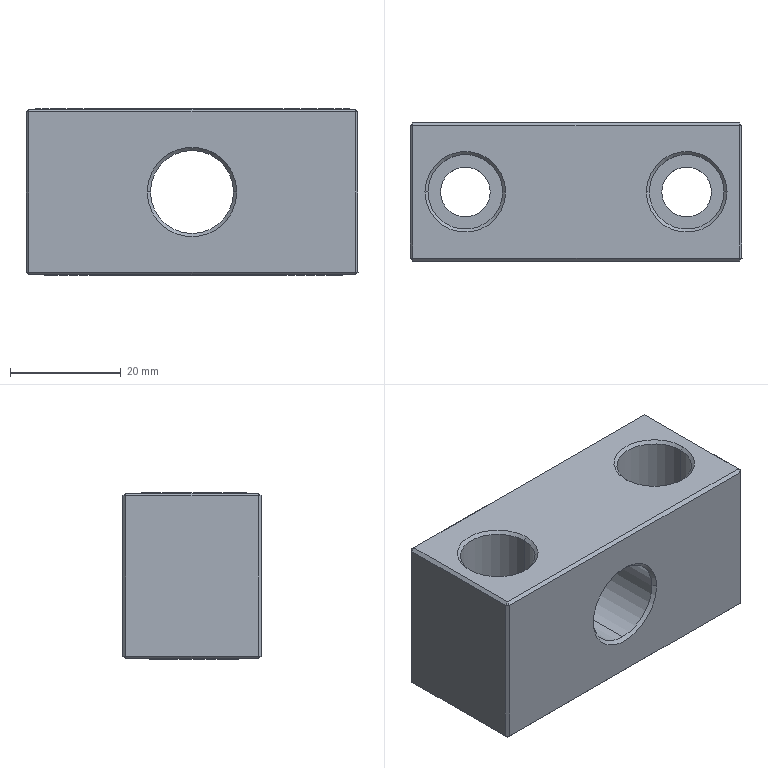Part | SolidWorks | features BaseBody 1 | 1 solid | 50 faces | box 60 x 25 x 30 mm | volume 34275 mm3 | plane 28 | cone 12 | cylinder 10 | commonest cylinder face diameters 9 x4 13.5 x4 15 x2
STEP:
#1=CARTESIAN_POINT('',(-7.5,-11.9,15.));
#2=VERTEX_POINT('',#1);
#3=CARTESIAN_POINT('',(0.,-11.9,7.5));
#4=VERTEX_POINT('',#3);
#5=CARTESIAN_POINT('',(0.,-11.9,15.));
#6=DIRECTION('',(0.,-1.,0.));
#7=DIRECTION('',(-1.,0.,0.));
#8=AXIS2_PLACEMENT_3D('',#5,#6,#7);
#9=CIRCLE('',#8,7.5);
#10=EDGE_CURVE('',#2,#4,#9,.T.);
#11=ORIENTED_EDGE('',*,*,#10,.F.);
#12=CARTESIAN_POINT('',(-8.1,-12.5,15.));
#13=VERTEX_POINT('',#12);
#14=CARTESIAN_POINT('',(-8.1,-12.5,15.));
#15=DIRECTION('',(-0.7071,-0.7071,0.));
#16=VECTOR('',#15,1000.);
#17=LINE('',#14,#16);
#18=EDGE_CURVE('',#2,#13,#17,.T.);
#19=ORIENTED_EDGE('',*,*,#18,.T.);
#20=CARTESIAN_POINT('',(8.1,-12.5,15.));
#21=VERTEX_POINT('',#20);
#22=CARTESIAN_POINT('',(0.,-12.5,15.));
#23=DIRECTION('',(0.,-1.,0.));
#24=DIRECTION('',(0.,0.,-1.));
#25=AXIS2_PLACEMENT_3D('',#22,#23,#24);
#26=CIRCLE('',#25,8.1);
#27=EDGE_CURVE('',#13,#21,#26,.T.);
#28=ORIENTED_EDGE('',*,*,#27,.T.);
#29=CARTESIAN_POINT('',(7.5,-11.9,15.));
#30=VERTEX_POINT('',#29);
#31=CARTESIAN_POINT('',(8.1,-12.5,15.));
#32=DIRECTION('',(0.7071,-0.7071,0.));
#33=VECTOR('',#32,1000.);
#34=LINE('',#31,#33);
#35=EDGE_CURVE('',#30,#21,#34,.T.);
#36=ORIENTED_EDGE('',*,*,#35,.F.);
#37=CARTESIAN_POINT('',(0.,-11.9,15.));
#38=DIRECTION('',(0.,-1.,0.));
#39=DIRECTION('',(-1.,0.,0.));
#40=AXIS2_PLACEMENT_3D('',#37,#38,#39);
#41=CIRCLE('',#40,7.5);
#42=EDGE_CURVE('',#4,#30,#41,.T.);
#43=ORIENTED_EDGE('',*,*,#42,.F.);
#44=EDGE_LOOP('',(#11,#19,#28,#36,#43));
#45=FACE_OUTER_BOUND('',#44,.T.);
#46=CARTESIAN_POINT('',(0.,-12.5,15.));
#47=DIRECTION('',(0.,-1.,0.));
#48=DIRECTION('',(1.,0.,0.));
#49=AXIS2_PLACEMENT_3D('',#46,#47,#48);
#50=CONICAL_SURFACE('',#49,8.1,0.7854);
#51=ADVANCED_FACE('',(#45),#50,.F.);
#52=CARTESIAN_POINT('',(0.,11.9,22.5));
#53=VERTEX_POINT('',#52);
#54=CARTESIAN_POINT('',(-7.5,11.9,15.));
#55=VERTEX_POINT('',#54);
#56=CARTESIAN_POINT('',(0.,11.9,15.));
#57=DIRECTION('',(0.,-1.,0.));
#58=DIRECTION('',(0.,0.,-1.));
#59=AXIS2_PLACEMENT_3D('',#56,#57,#58);
#60=CIRCLE('',#59,7.5);
#61=EDGE_CURVE('',#53,#55,#60,.T.);
#62=ORIENTED_EDGE('',*,*,#61,.F.);
#63=CARTESIAN_POINT('',(0.,-11.9,22.5));
#64=VERTEX_POINT('',#63);
#65=CARTESIAN_POINT('',(0.,12.5,22.5));
#66=DIRECTION('',(0.,-1.,0.));
#67=VECTOR('',#66,1000.);
#68=LINE('',#65,#67);
#69=EDGE_CURVE('',#53,#64,#68,.T.);
#70=ORIENTED_EDGE('',*,*,#69,.T.);
#71=CARTESIAN_POINT('',(0.,-11.9,15.));
#72=DIRECTION('',(0.,-1.,0.));
#73=DIRECTION('',(-1.,0.,0.));
#74=AXIS2_PLACEMENT_3D('',#71,#72,#73);
#75=CIRCLE('',#74,7.5);
#76=EDGE_CURVE('',#64,#2,#75,.T.);
#77=ORIENTED_EDGE('',*,*,#76,.T.);
#78=ORIENTED_EDGE('',*,*,#10,.T.);
#79=CARTESIAN_POINT('',(0.,11.9,7.5));
#80=VERTEX_POINT('',#79);
#81=CARTESIAN_POINT('',(0.,12.5,7.5));
#82=DIRECTION('',(0.,-1.,0.));
#83=VECTOR('',#82,1000.);
#84=LINE('',#81,#83);
#85=EDGE_CURVE('',#80,#4,#84,.T.);
#86=ORIENTED_EDGE('',*,*,#85,.F.);
#87=CARTESIAN_POINT('',(0.,11.9,15.));
#88=DIRECTION('',(0.,-1.,0.));
#89=DIRECTION('',(0.,0.,-1.));
#90=AXIS2_PLACEMENT_3D('',#87,#88,#89);
#91=CIRCLE('',#90,7.5);
#92=EDGE_CURVE('',#55,#80,#91,.T.);
#93=ORIENTED_EDGE('',*,*,#92,.F.);
#94=EDGE_LOOP('',(#62,#70,#77,#78,#86,#93));
#95=FACE_OUTER_BOUND('',#94,.T.);
#96=CARTESIAN_POINT('',(0.,12.5,15.));
#97=DIRECTION('',(0.,-1.,0.));
#98=DIRECTION('',(0.,0.,-1.));
#99=AXIS2_PLACEMENT_3D('',#96,#97,#98);
#100=CYLINDRICAL_SURFACE('',#99,7.5);
#101=ADVANCED_FACE('',(#95),#100,.F.);
#102=ORIENTED_EDGE('',*,*,#92,.T.);
#103=CARTESIAN_POINT('',(7.5,11.9,15.));
#104=VERTEX_POINT('',#103);
#105=CARTESIAN_POINT('',(0.,11.9,15.));
#106=DIRECTION('',(0.,-1.,0.));
#107=DIRECTION('',(0.,0.,-1.));
#108=AXIS2_PLACEMENT_3D('',#105,#106,#107);
#109=CIRCLE('',#108,7.5);
#110=EDGE_CURVE('',#80,#104,#109,.T.);
#111=ORIENTED_EDGE('',*,*,#110,.T.);
#112=CARTESIAN_POINT('',(8.1,12.5,15.));
#113=VERTEX_POINT('',#112);
#114=CARTESIAN_POINT('',(8.1,12.5,15.));
#115=DIRECTION('',(0.7071,0.7071,0.));
#116=VECTOR('',#115,1000.);
#117=LINE('',#114,#116);
#118=EDGE_CURVE('',#104,#113,#117,.T.);
#119=ORIENTED_EDGE('',*,*,#118,.T.);
#120=CARTESIAN_POINT('',(-8.1,12.5,15.));
#121=VERTEX_POINT('',#120);
#122=CARTESIAN_POINT('',(0.,12.5,15.));
#123=DIRECTION('',(0.,-1.,0.));
#124=DIRECTION('',(-1.,0.,0.));
#125=AXIS2_PLACEMENT_3D('',#122,#123,#124);
#126=CIRCLE('',#125,8.1);
#127=EDGE_CURVE('',#121,#113,#126,.T.);
#128=ORIENTED_EDGE('',*,*,#127,.F.);
#129=CARTESIAN_POINT('',(-8.1,12.5,15.));
#130=DIRECTION('',(-0.7071,0.7071,0.));
#131=VECTOR('',#130,1000.);
#132=LINE('',#129,#131);
#133=EDGE_CURVE('',#55,#121,#132,.T.);
#134=ORIENTED_EDGE('',*,*,#133,.F.);
#135=EDGE_LOOP('',(#102,#111,#119,#128,#134));
#136=FACE_OUTER_BOUND('',#135,.T.);
#137=CARTESIAN_POINT('',(0.,12.5,15.));
#138=DIRECTION('',(0.,1.,0.));
#139=DIRECTION('',(-1.,0.,0.));
#140=AXIS2_PLACEMENT_3D('',#137,#138,#139);
#141=CONICAL_SURFACE('',#140,8.1,0.7854);
#142=ADVANCED_FACE('',(#136),#141,.F.);
#143=CARTESIAN_POINT('',(-15.5,0.,0.54));
#144=VERTEX_POINT('',#143);
#145=CARTESIAN_POINT('',(-24.5,0.,0.54));
#146=VERTEX_POINT('',#145);
#147=CARTESIAN_POINT('',(-20.,0.,0.54));
#148=DIRECTION('',(0.,0.,-1.));
#149=DIRECTION('',(-1.,0.,0.));
#150=AXIS2_PLACEMENT_3D('',#147,#148,#149);
#151=CIRCLE('',#150,4.5);
#152=EDGE_CURVE('',#144,#146,#151,.T.);
#153=ORIENTED_EDGE('',*,*,#152,.F.);
#154=CARTESIAN_POINT('',(-14.96,0.,0.));
#155=VERTEX_POINT('',#154);
#156=CARTESIAN_POINT('',(-14.96,0.,0.));
#157=DIRECTION('',(0.7071,0.,-0.7071));
#158=VECTOR('',#157,1000.);
#159=LINE('',#156,#158);
#160=EDGE_CURVE('',#144,#155,#159,.T.);
#161=ORIENTED_EDGE('',*,*,#160,.T.);
#162=CARTESIAN_POINT('',(-25.04,0.,0.));
#163=VERTEX_POINT('',#162);
#164=CARTESIAN_POINT('',(-20.,0.,0.));
#165=DIRECTION('',(0.,0.,1.));
#166=DIRECTION('',(-1.,0.,0.));
#167=AXIS2_PLACEMENT_3D('',#164,#165,#166);
#168=CIRCLE('',#167,5.04);
#169=EDGE_CURVE('',#163,#155,#168,.T.);
#170=ORIENTED_EDGE('',*,*,#169,.F.);
#171=CARTESIAN_POINT('',(-25.04,0.,0.));
#172=DIRECTION('',(-0.7071,0.,-0.7071));
#173=VECTOR('',#172,1000.);
#174=LINE('',#171,#173);
#175=EDGE_CURVE('',#146,#163,#174,.T.);
#176=ORIENTED_EDGE('',*,*,#175,.F.);
#177=EDGE_LOOP('',(#153,#161,#170,#176));
#178=FACE_OUTER_BOUND('',#177,.T.);
#179=CARTESIAN_POINT('',(-20.,0.,0.));
#180=DIRECTION('',(0.,0.,-1.));
#181=DIRECTION('',(-1.,0.,0.));
#182=AXIS2_PLACEMENT_3D('',#179,#180,#181);
#183=CONICAL_SURFACE('',#182,5.04,0.7854);
#184=ADVANCED_FACE('',(#178),#183,.F.);
#185=CARTESIAN_POINT('',(24.5,0.,0.54));
#186=VERTEX_POINT('',#185);
#187=CARTESIAN_POINT('',(15.5,0.,0.54));
#188=VERTEX_POINT('',#187);
#189=CARTESIAN_POINT('',(20.,0.,0.54));
#190=DIRECTION('',(0.,0.,-1.));
#191=DIRECTION('',(-1.,0.,0.));
#192=AXIS2_PLACEMENT_3D('',#189,#190,#191);
#193=CIRCLE('',#192,4.5);
#194=EDGE_CURVE('',#186,#188,#193,.T.);
#195=ORIENTED_EDGE('',*,*,#194,.F.);
#196=CARTESIAN_POINT('',(25.04,0.,0.));
#197=VERTEX_POINT('',#196);
#198=CARTESIAN_POINT('',(25.04,0.,0.));
#199=DIRECTION('',(0.7071,0.,-0.7071));
#200=VECTOR('',#199,1000.);
#201=LINE('',#198,#200);
#202=EDGE_CURVE('',#186,#197,#201,.T.);
#203=ORIENTED_EDGE('',*,*,#202,.T.);
#204=CARTESIAN_POINT('',(14.96,0.,0.));
#205=VERTEX_POINT('',#204);
#206=CARTESIAN_POINT('',(20.,0.,0.));
#207=DIRECTION('',(0.,0.,1.));
#208=DIRECTION('',(-1.,0.,0.));
#209=AXIS2_PLACEMENT_3D('',#206,#207,#208);
#210=CIRCLE('',#209,5.04);
#211=EDGE_CURVE('',#205,#197,#210,.T.);
#212=ORIENTED_EDGE('',*,*,#211,.F.);
#213=CARTESIAN_POINT('',(14.96,0.,0.));
#214=DIRECTION('',(-0.7071,0.,-0.7071));
#215=VECTOR('',#214,1000.);
#216=LINE('',#213,#215);
#217=EDGE_CURVE('',#188,#205,#216,.T.);
#218=ORIENTED_EDGE('',*,*,#217,.F.);
#219=EDGE_LOOP('',(#195,#203,#212,#218));
#220=FACE_OUTER_BOUND('',#219,.T.);
#221=CARTESIAN_POINT('',(20.,0.,0.));
#222=DIRECTION('',(0.,0.,-1.));
#223=DIRECTION('',(-1.,0.,0.));
#224=AXIS2_PLACEMENT_3D('',#221,#222,#223);
#225=CONICAL_SURFACE('',#224,5.04,0.7854);
#226=ADVANCED_FACE('',(#220),#225,.F.);
#227=CARTESIAN_POINT('',(13.25,0.,29.46));
#228=VERTEX_POINT('',#227);
#229=CARTESIAN_POINT('',(26.75,0.,29.46));
#230=VERTEX_POINT('',#229);
#231=CARTESIAN_POINT('',(20.,0.,29.46));
#232=DIRECTION('',(0.,0.,1.));
#233=DIRECTION('',(-1.,0.,0.));
#234=AXIS2_PLACEMENT_3D('',#231,#232,#233);
#235=CIRCLE('',#234,6.75);
#236=EDGE_CURVE('',#228,#230,#235,.T.);
#237=ORIENTED_EDGE('',*,*,#236,.F.);
#238=CARTESIAN_POINT('',(12.71,0.,30.));
#239=VERTEX_POINT('',#238);
#240=CARTESIAN_POINT('',(12.71,0.,30.));
#241=DIRECTION('',(-0.7071,0.,0.7071));
#242=VECTOR('',#241,1000.);
#243=LINE('',#240,#242);
#244=EDGE_CURVE('',#228,#239,#243,.T.);
#245=ORIENTED_EDGE('',*,*,#244,.T.);
#246=CARTESIAN_POINT('',(27.29,0.,30.));
#247=VERTEX_POINT('',#246);
#248=CARTESIAN_POINT('',(20.,0.,30.));
#249=DIRECTION('',(0.,0.,1.));
#250=DIRECTION('',(1.,0.,0.));
#251=AXIS2_PLACEMENT_3D('',#248,#249,#250);
#252=CIRCLE('',#251,7.29);
#253=EDGE_CURVE('',#239,#247,#252,.T.);
#254=ORIENTED_EDGE('',*,*,#253,.T.);
#255=CARTESIAN_POINT('',(27.29,0.,30.));
#256=DIRECTION('',(0.7071,0.,0.7071));
#257=VECTOR('',#256,1000.);
#258=LINE('',#255,#257);
#259=EDGE_CURVE('',#230,#247,#258,.T.);
#260=ORIENTED_EDGE('',*,*,#259,.F.);
#261=EDGE_LOOP('',(#237,#245,#254,#260));
#262=FACE_OUTER_BOUND('',#261,.T.);
#263=CARTESIAN_POINT('',(20.,0.,30.));
#264=DIRECTION('',(0.,0.,1.));
#265=DIRECTION('',(1.,0.,0.));
#266=AXIS2_PLACEMENT_3D('',#263,#264,#265);
#267=CONICAL_SURFACE('',#266,7.29,0.7854);
#268=ADVANCED_FACE('',(#262),#267,.F.);
#269=CARTESIAN_POINT('',(-26.75,0.,29.46));
#270=VERTEX_POINT('',#269);
#271=CARTESIAN_POINT('',(-13.25,0.,29.46));
#272=VERTEX_POINT('',#271);
#273=CARTESIAN_POINT('',(-20.,0.,29.46));
#274=DIRECTION('',(0.,0.,1.));
#275=DIRECTION('',(-1.,0.,0.));
#276=AXIS2_PLACEMENT_3D('',#273,#274,#275);
#277=CIRCLE('',#276,6.75);
#278=EDGE_CURVE('',#270,#272,#277,.T.);
#279=ORIENTED_EDGE('',*,*,#278,.F.);
#280=CARTESIAN_POINT('',(-27.29,0.,30.));
#281=VERTEX_POINT('',#280);
#282=CARTESIAN_POINT('',(-27.29,0.,30.));
#283=DIRECTION('',(-0.7071,0.,0.7071));
#284=VECTOR('',#283,1000.);
#285=LINE('',#282,#284);
#286=EDGE_CURVE('',#270,#281,#285,.T.);
#287=ORIENTED_EDGE('',*,*,#286,.T.);
#288=CARTESIAN_POINT('',(-12.71,0.,30.));
#289=VERTEX_POINT('',#288);
#290=CARTESIAN_POINT('',(-20.,0.,30.));
#291=DIRECTION('',(0.,0.,1.));
#292=DIRECTION('',(1.,0.,0.));
#293=AXIS2_PLACEMENT_3D('',#290,#291,#292);
#294=CIRCLE('',#293,7.29);
#295=EDGE_CURVE('',#281,#289,#294,.T.);
#296=ORIENTED_EDGE('',*,*,#295,.T.);
#297=CARTESIAN_POINT('',(-12.71,0.,30.));
#298=DIRECTION('',(0.7071,0.,0.7071));
#299=VECTOR('',#298,1000.);
#300=LINE('',#297,#299);
#301=EDGE_CURVE('',#272,#289,#300,.T.);
#302=ORIENTED_EDGE('',*,*,#301,.F.);
#303=EDGE_LOOP('',(#279,#287,#296,#302));
#304=FACE_OUTER_BOUND('',#303,.T.);
#305=CARTESIAN_POINT('',(-20.,0.,30.));
#306=DIRECTION('',(0.,0.,1.));
#307=DIRECTION('',(1.,0.,0.));
#308=AXIS2_PLACEMENT_3D('',#305,#306,#307);
#309=CONICAL_SURFACE('',#308,7.29,0.7854);
#310=ADVANCED_FACE('',(#304),#309,.F.);
#311=ORIENTED_EDGE('',*,*,#152,.T.);
#312=CARTESIAN_POINT('',(-24.5,0.,15.));
#313=VERTEX_POINT('',#312);
#314=CARTESIAN_POINT('',(-24.5,0.,0.));
#315=DIRECTION('',(0.,0.,1.));
#316=VECTOR('',#315,1000.);
#317=LINE('',#314,#316);
#318=EDGE_CURVE('',#146,#313,#317,.T.);
#319=ORIENTED_EDGE('',*,*,#318,.T.);
#320=CARTESIAN_POINT('',(-15.5,0.,15.));
#321=VERTEX_POINT('',#320);
#322=CARTESIAN_POINT('',(-20.,0.,15.));
#323=DIRECTION('',(0.,0.,-1.));
#324=DIRECTION('',(1.,0.,0.));
#325=AXIS2_PLACEMENT_3D('',#322,#323,#324);
#326=CIRCLE('',#325,4.5);
#327=EDGE_CURVE('',#321,#313,#326,.T.);
#328=ORIENTED_EDGE('',*,*,#327,.F.);
#329=CARTESIAN_POINT('',(-15.5,0.,0.));
#330=DIRECTION('',(0.,0.,1.));
#331=VECTOR('',#330,1000.);
#332=LINE('',#329,#331);
#333=EDGE_CURVE('',#144,#321,#332,.T.);
#334=ORIENTED_EDGE('',*,*,#333,.F.);
#335=EDGE_LOOP('',(#311,#319,#328,#334));
#336=FACE_OUTER_BOUND('',#335,.T.);
#337=CARTESIAN_POINT('',(-20.,0.,0.));
#338=DIRECTION('',(0.,0.,1.));
#339=DIRECTION('',(1.,0.,0.));
#340=AXIS2_PLACEMENT_3D('',#337,#338,#339);
#341=CYLINDRICAL_SURFACE('',#340,4.5);
#342=ADVANCED_FACE('',(#336),#341,.F.);
#343=ORIENTED_EDGE('',*,*,#194,.T.);
#344=CARTESIAN_POINT('',(15.5,0.,15.));
#345=VERTEX_POINT('',#344);
#346=CARTESIAN_POINT('',(15.5,0.,0.));
#347=DIRECTION('',(0.,0.,1.));
#348=VECTOR('',#347,1000.);
#349=LINE('',#346,#348);
#350=EDGE_CURVE('',#188,#345,#349,.T.);
#351=ORIENTED_EDGE('',*,*,#350,.T.);
#352=CARTESIAN_POINT('',(24.5,0.,15.));
#353=VERTEX_POINT('',#352);
#354=CARTESIAN_POINT('',(20.,0.,15.));
#355=DIRECTION('',(0.,0.,-1.));
#356=DIRECTION('',(1.,0.,0.));
#357=AXIS2_PLACEMENT_3D('',#354,#355,#356);
#358=CIRCLE('',#357,4.5);
#359=EDGE_CURVE('',#353,#345,#358,.T.);
#360=ORIENTED_EDGE('',*,*,#359,.F.);
#361=CARTESIAN_POINT('',(24.5,0.,0.));
#362=DIRECTION('',(0.,0.,1.));
#363=VECTOR('',#362,1000.);
#364=LINE('',#361,#363);
#365=EDGE_CURVE('',#186,#353,#364,.T.);
#366=ORIENTED_EDGE('',*,*,#365,.F.);
#367=EDGE_LOOP('',(#343,#351,#360,#366));
#368=FACE_OUTER_BOUND('',#367,.T.);
#369=CARTESIAN_POINT('',(20.,0.,0.));
#370=DIRECTION('',(0.,0.,1.));
#371=DIRECTION('',(1.,0.,0.));
#372=AXIS2_PLACEMENT_3D('',#369,#370,#371);
#373=CYLINDRICAL_SURFACE('',#372,4.5);
#374=ADVANCED_FACE('',(#368),#373,.F.);
#375=CARTESIAN_POINT('',(13.25,0.,15.));
#376=VERTEX_POINT('',#375);
#377=CARTESIAN_POINT('',(26.75,0.,15.));
#378=VERTEX_POINT('',#377);
#379=CARTESIAN_POINT('',(20.,0.,15.));
#380=DIRECTION('',(0.,0.,1.));
#381=DIRECTION('',(1.,0.,0.));
#382=AXIS2_PLACEMENT_3D('',#379,#380,#381);
#383=CIRCLE('',#382,6.75);
#384=EDGE_CURVE('',#376,#378,#383,.T.);
#385=ORIENTED_EDGE('',*,*,#384,.F.);
#386=CARTESIAN_POINT('',(13.25,0.,15.));
#387=DIRECTION('',(0.,0.,1.));
#388=VECTOR('',#387,1000.);
#389=LINE('',#386,#388);
#390=EDGE_CURVE('',#376,#228,#389,.T.);
#391=ORIENTED_EDGE('',*,*,#390,.T.);
#392=ORIENTED_EDGE('',*,*,#236,.T.);
#393=CARTESIAN_POINT('',(26.75,0.,15.));
#394=DIRECTION('',(0.,0.,1.));
#395=VECTOR('',#394,1000.);
#396=LINE('',#393,#395);
#397=EDGE_CURVE('',#378,#230,#396,.T.);
#398=ORIENTED_EDGE('',*,*,#397,.F.);
#399=EDGE_LOOP('',(#385,#391,#392,#398));
#400=FACE_OUTER_BOUND('',#399,.T.);
#401=CARTESIAN_POINT('',(20.,0.,15.));
#402=DIRECTION('',(0.,0.,1.));
#403=DIRECTION('',(1.,0.,0.));
#404=AXIS2_PLACEMENT_3D('',#401,#402,#403);
#405=CYLINDRICAL_SURFACE('',#404,6.75);
#406=ADVANCED_FACE('',(#400),#405,.F.);
#407=CARTESIAN_POINT('',(-26.75,0.,15.));
#408=VERTEX_POINT('',#407);
#409=CARTESIAN_POINT('',(-13.25,0.,15.));
#410=VERTEX_POINT('',#409);
#411=CARTESIAN_POINT('',(-20.,0.,15.));
#412=DIRECTION('',(0.,0.,1.));
#413=DIRECTION('',(1.,0.,0.));
#414=AXIS2_PLACEMENT_3D('',#411,#412,#413);
#415=CIRCLE('',#414,6.75);
#416=EDGE_CURVE('',#408,#410,#415,.T.);
#417=ORIENTED_EDGE('',*,*,#416,.F.);
#418=CARTESIAN_POINT('',(-26.75,0.,15.));
#419=DIRECTION('',(0.,0.,1.));
#420=VECTOR('',#419,1000.);
#421=LINE('',#418,#420);
#422=EDGE_CURVE('',#408,#270,#421,.T.);
#423=ORIENTED_EDGE('',*,*,#422,.T.);
#424=ORIENTED_EDGE('',*,*,#278,.T.);
#425=CARTESIAN_POINT('',(-13.25,0.,15.));
#426=DIRECTION('',(0.,0.,1.));
#427=VECTOR('',#426,1000.);
#428=LINE('',#425,#427);
#429=EDGE_CURVE('',#410,#272,#428,.T.);
#430=ORIENTED_EDGE('',*,*,#429,.F.);
#431=EDGE_LOOP('',(#417,#423,#424,#430));
#432=FACE_OUTER_BOUND('',#431,.T.);
#433=CARTESIAN_POINT('',(-20.,0.,15.));
#434=DIRECTION('',(0.,0.,1.));
#435=DIRECTION('',(1.,0.,0.));
#436=AXIS2_PLACEMENT_3D('',#433,#434,#435);
#437=CYLINDRICAL_SURFACE('',#436,6.75);
#438=ADVANCED_FACE('',(#432),#437,.F.);
#439=CARTESIAN_POINT('',(0.,-12.5,15.));
#440=DIRECTION('',(0.,-1.,0.));
#441=DIRECTION('',(0.,0.,-1.));
#442=AXIS2_PLACEMENT_3D('',#439,#440,#441);
#443=CIRCLE('',#442,8.1);
#444=EDGE_CURVE('',#21,#13,#443,.T.);
#445=ORIENTED_EDGE('',*,*,#444,.F.);
#446=ORIENTED_EDGE('',*,*,#27,.F.);
#447=EDGE_LOOP('',(#445,#446));
#448=FACE_BOUND('',#447,.T.);
#449=CARTESIAN_POINT('',(29.46,-12.5,29.46));
#450=VERTEX_POINT('',#449);
#451=CARTESIAN_POINT('',(29.46,-12.5,0.54));
#452=VERTEX_POINT('',#451);
#453=CARTESIAN_POINT('',(29.46,-12.5,30.));
#454=DIRECTION('',(0.,0.,-1.));
#455=VECTOR('',#454,1000.);
#456=LINE('',#453,#455);
#457=EDGE_CURVE('',#450,#452,#456,.T.);
#458=ORIENTED_EDGE('',*,*,#457,.F.);
#459=CARTESIAN_POINT('',(-29.46,-12.5,29.46));
#460=VERTEX_POINT('',#459);
#461=CARTESIAN_POINT('',(30.,-12.5,29.46));
#462=DIRECTION('',(1.,0.,0.));
#463=VECTOR('',#462,1000.);
#464=LINE('',#461,#463);
#465=EDGE_CURVE('',#460,#450,#464,.T.);
#466=ORIENTED_EDGE('',*,*,#465,.F.);
#467=CARTESIAN_POINT('',(-29.46,-12.5,0.54));
#468=VERTEX_POINT('',#467);
#469=CARTESIAN_POINT('',(-29.46,-12.5,30.));
#470=DIRECTION('',(0.,0.,1.));
#471=VECTOR('',#470,1000.);
#472=LINE('',#469,#471);
#473=EDGE_CURVE('',#468,#460,#472,.T.);
#474=ORIENTED_EDGE('',*,*,#473,.F.);
#475=CARTESIAN_POINT('',(30.,-12.5,0.54));
#476=DIRECTION('',(-1.,0.,0.));
#477=VECTOR('',#476,1000.);
#478=LINE('',#475,#477);
#479=EDGE_CURVE('',#452,#468,#478,.T.);
#480=ORIENTED_EDGE('',*,*,#479,.F.);
#481=EDGE_LOOP('',(#458,#466,#474,#480));
#482=FACE_OUTER_BOUND('',#481,.T.);
#483=CARTESIAN_POINT('',(30.,-12.5,30.));
#484=DIRECTION('',(0.,1.,0.));
#485=DIRECTION('',(-1.,0.,0.));
#486=AXIS2_PLACEMENT_3D('',#483,#484,#485);
#487=PLANE('',#486);
#488=ADVANCED_FACE('',(#448,#482),#487,.F.);
#489=ORIENTED_EDGE('',*,*,#18,.F.);
#490=ORIENTED_EDGE('',*,*,#76,.F.);
#491=CARTESIAN_POINT('',(0.,-11.9,15.));
#492=DIRECTION('',(0.,-1.,0.));
#493=DIRECTION('',(-1.,0.,0.));
#494=AXIS2_PLACEMENT_3D('',#491,#492,#493);
#495=CIRCLE('',#494,7.5);
#496=EDGE_CURVE('',#30,#64,#495,.T.);
#497=ORIENTED_EDGE('',*,*,#496,.F.);
#498=ORIENTED_EDGE('',*,*,#35,.T.);
#499=ORIENTED_EDGE('',*,*,#444,.T.);
#500=EDGE_LOOP('',(#489,#490,#497,#498,#499));
#501=FACE_OUTER_BOUND('',#500,.T.);
#502=CARTESIAN_POINT('',(0.,-12.5,15.));
#503=DIRECTION('',(0.,-1.,0.));
#504=DIRECTION('',(1.,0.,0.));
#505=AXIS2_PLACEMENT_3D('',#502,#503,#504);
#506=CONICAL_SURFACE('',#505,8.1,0.7854);
#507=ADVANCED_FACE('',(#501),#506,.F.);
#508=CARTESIAN_POINT('',(29.46,-11.96,0.));
#509=VERTEX_POINT('',#508);
#510=CARTESIAN_POINT('',(29.46,-12.5,0.54));
#511=DIRECTION('',(0.,-0.7071,0.7071));
#512=VECTOR('',#511,1000.);
#513=LINE('',#510,#512);
#514=EDGE_CURVE('',#509,#452,#513,.T.);
#515=ORIENTED_EDGE('',*,*,#514,.T.);
#516=ORIENTED_EDGE('',*,*,#479,.T.);
#517=CARTESIAN_POINT('',(-29.46,-11.96,0.));
#518=VERTEX_POINT('',#517);
#519=CARTESIAN_POINT('',(-29.46,-12.5,0.54));
#520=DIRECTION('',(0.,0.7071,-0.7071));
#521=VECTOR('',#520,1000.);
#522=LINE('',#519,#521);
#523=EDGE_CURVE('',#468,#518,#522,.T.);
#524=ORIENTED_EDGE('',*,*,#523,.T.);
#525=CARTESIAN_POINT('',(30.,-11.96,0.));
#526=DIRECTION('',(1.,0.,0.));
#527=VECTOR('',#526,1000.);
#528=LINE('',#525,#527);
#529=EDGE_CURVE('',#518,#509,#528,.T.);
#530=ORIENTED_EDGE('',*,*,#529,.T.);
#531=EDGE_LOOP('',(#515,#516,#524,#530));
#532=FACE_OUTER_BOUND('',#531,.T.);
#533=CARTESIAN_POINT('',(30.,-12.5,0.54));
#534=DIRECTION('',(0.,-0.7071,-0.7071));
#535=DIRECTION('',(0.,0.7071,-0.7071));
#536=AXIS2_PLACEMENT_3D('',#533,#534,#535);
#537=PLANE('',#536);
#538=ADVANCED_FACE('',(#532),#537,.T.);
#539=ORIENTED_EDGE('',*,*,#457,.T.);
#540=CARTESIAN_POINT('',(30.,-11.96,0.54));
#541=VERTEX_POINT('',#540);
#542=CARTESIAN_POINT('',(30.,-11.96,0.54));
#543=DIRECTION('',(-0.7071,-0.7071,0.));
#544=VECTOR('',#543,1000.);
#545=LINE('',#542,#544);
#546=EDGE_CURVE('',#541,#452,#545,.T.);
#547=ORIENTED_EDGE('',*,*,#546,.F.);
#548=CARTESIAN_POINT('',(30.,-11.96,29.46));
#549=VERTEX_POINT('',#548);
#550=CARTESIAN_POINT('',(30.,-11.96,30.));
#551=DIRECTION('',(0.,0.,-1.));
#552=VECTOR('',#551,1000.);
#553=LINE('',#550,#552);
#554=EDGE_CURVE('',#549,#541,#553,.T.);
#555=ORIENTED_EDGE('',*,*,#554,.F.);
#556=CARTESIAN_POINT('',(30.,-11.96,29.46));
#557=DIRECTION('',(0.7071,0.7071,0.));
#558=VECTOR('',#557,1000.);
#559=LINE('',#556,#558);
#560=EDGE_CURVE('',#450,#549,#559,.T.);
#561=ORIENTED_EDGE('',*,*,#560,.F.);
#562=EDGE_LOOP('',(#539,#547,#555,#561));
#563=FACE_OUTER_BOUND('',#562,.T.);
#564=CARTESIAN_POINT('',(30.,-11.96,30.));
#565=DIRECTION('',(-0.7071,0.7071,0.));
#566=DIRECTION('',(-0.7071,-0.7071,0.));
#567=AXIS2_PLACEMENT_3D('',#564,#565,#566);
#568=PLANE('',#567);
#569=ADVANCED_FACE('',(#563),#568,.F.);
#570=ORIENTED_EDGE('',*,*,#465,.T.);
#571=CARTESIAN_POINT('',(29.46,-11.96,30.));
#572=VERTEX_POINT('',#571);
#573=CARTESIAN_POINT('',(29.46,-11.96,30.));
#574=DIRECTION('',(0.,-0.7071,-0.7071));
#575=VECTOR('',#574,1000.);
#576=LINE('',#573,#575);
#577=EDGE_CURVE('',#572,#450,#576,.T.);
#578=ORIENTED_EDGE('',*,*,#577,.F.);
#579=CARTESIAN_POINT('',(-29.46,-11.96,30.));
#580=VERTEX_POINT('',#579);
#581=CARTESIAN_POINT('',(0.,-11.96,30.));
#582=DIRECTION('',(1.,0.,0.));
#583=VECTOR('',#582,1000.);
#584=LINE('',#581,#583);
#585=EDGE_CURVE('',#580,#572,#584,.T.);
#586=ORIENTED_EDGE('',*,*,#585,.F.);
#587=CARTESIAN_POINT('',(-29.46,-11.96,30.));
#588=DIRECTION('',(0.,0.7071,0.7071));
#589=VECTOR('',#588,1000.);
#590=LINE('',#587,#589);
#591=EDGE_CURVE('',#460,#580,#590,.T.);
#592=ORIENTED_EDGE('',*,*,#591,.F.);
#593=EDGE_LOOP('',(#570,#578,#586,#592));
#594=FACE_OUTER_BOUND('',#593,.T.);
#595=CARTESIAN_POINT('',(0.,-11.96,30.));
#596=DIRECTION('',(0.,0.7071,-0.7071));
#597=DIRECTION('',(0.,0.7071,0.7071));
#598=AXIS2_PLACEMENT_3D('',#595,#596,#597);
#599=PLANE('',#598);
#600=ADVANCED_FACE('',(#594),#599,.F.);
#601=CARTESIAN_POINT('',(-30.,-11.96,0.54));
#602=VERTEX_POINT('',#601);
#603=CARTESIAN_POINT('',(-30.,-11.96,29.46));
#604=VERTEX_POINT('',#603);
#605=CARTESIAN_POINT('',(-30.,-11.96,30.));
#606=DIRECTION('',(0.,0.,1.));
#607=VECTOR('',#606,1000.);
#608=LINE('',#605,#607);
#609=EDGE_CURVE('',#602,#604,#608,.T.);
#610=ORIENTED_EDGE('',*,*,#609,.F.);
#611=CARTESIAN_POINT('',(-29.46,-12.5,0.54));
#612=DIRECTION('',(-0.7071,0.7071,0.));
#613=VECTOR('',#612,1000.);
#614=LINE('',#611,#613);
#615=EDGE_CURVE('',#468,#602,#614,.T.);
#616=ORIENTED_EDGE('',*,*,#615,.F.);
#617=ORIENTED_EDGE('',*,*,#473,.T.);
#618=CARTESIAN_POINT('',(-29.46,-12.5,29.46));
#619=DIRECTION('',(0.7071,-0.7071,0.));
#620=VECTOR('',#619,1000.);
#621=LINE('',#618,#620);
#622=EDGE_CURVE('',#604,#460,#621,.T.);
#623=ORIENTED_EDGE('',*,*,#622,.F.);
#624=EDGE_LOOP('',(#610,#616,#617,#623));
#625=FACE_OUTER_BOUND('',#624,.T.);
#626=CARTESIAN_POINT('',(-29.46,-12.5,30.));
#627=DIRECTION('',(0.7071,0.7071,0.));
#628=DIRECTION('',(-0.7071,0.7071,0.));
#629=AXIS2_PLACEMENT_3D('',#626,#627,#628);
#630=PLANE('',#629);
#631=ADVANCED_FACE('',(#625),#630,.F.);
#632=ORIENTED_EDGE('',*,*,#69,.F.);
#633=CARTESIAN_POINT('',(0.,11.9,15.));
#634=DIRECTION('',(0.,-1.,0.));
#635=DIRECTION('',(0.,0.,-1.));
#636=AXIS2_PLACEMENT_3D('',#633,#634,#635);
#637=CIRCLE('',#636,7.5);
#638=EDGE_CURVE('',#104,#53,#637,.T.);
#639=ORIENTED_EDGE('',*,*,#638,.F.);
#640=ORIENTED_EDGE('',*,*,#110,.F.);
#641=ORIENTED_EDGE('',*,*,#85,.T.);
#642=ORIENTED_EDGE('',*,*,#42,.T.);
#643=ORIENTED_EDGE('',*,*,#496,.T.);
#644=EDGE_LOOP('',(#632,#639,#640,#641,#642,#643));
#645=FACE_OUTER_BOUND('',#644,.T.);
#646=CARTESIAN_POINT('',(0.,12.5,15.));
#647=DIRECTION('',(0.,-1.,0.));
#648=DIRECTION('',(0.,0.,-1.));
#649=AXIS2_PLACEMENT_3D('',#646,#647,#648);
#650=CYLINDRICAL_SURFACE('',#649,7.5);
#651=ADVANCED_FACE('',(#645),#650,.F.);
#652=CARTESIAN_POINT('',(30.,-11.96,0.54));
#653=DIRECTION('',(-0.7071,0.,-0.7071));
#654=VECTOR('',#653,1000.);
#655=LINE('',#652,#654);
#656=EDGE_CURVE('',#541,#509,#655,.T.);
#657=ORIENTED_EDGE('',*,*,#656,.F.);
#658=ORIENTED_EDGE('',*,*,#546,.T.);
#659=ORIENTED_EDGE('',*,*,#514,.F.);
#660=EDGE_LOOP('',(#657,#658,#659));
#661=FACE_OUTER_BOUND('',#660,.T.);
#662=CARTESIAN_POINT('',(30.,-11.96,0.54));
#663=DIRECTION('',(0.5774,-0.5774,-0.5774));
#664=DIRECTION('',(-0.7071,0.,-0.7071));
#665=AXIS2_PLACEMENT_3D('',#662,#663,#664);
#666=PLANE('',#665);
#667=ADVANCED_FACE('',(#661),#666,.T.);
#668=ORIENTED_EDGE('',*,*,#169,.T.);
#669=CARTESIAN_POINT('',(-20.,0.,0.));
#670=DIRECTION('',(0.,0.,1.));
#671=DIRECTION('',(-1.,0.,0.));
#672=AXIS2_PLACEMENT_3D('',#669,#670,#671);
#673=CIRCLE('',#672,5.04);
#674=EDGE_CURVE('',#155,#163,#673,.T.);
#675=ORIENTED_EDGE('',*,*,#674,.T.);
#676=EDGE_LOOP('',(#668,#675));
#677=FACE_BOUND('',#676,.T.);
#678=ORIENTED_EDGE('',*,*,#211,.T.);
#679=CARTESIAN_POINT('',(20.,0.,0.));
#680=DIRECTION('',(0.,0.,1.));
#681=DIRECTION('',(-1.,0.,0.));
#682=AXIS2_PLACEMENT_3D('',#679,#680,#681);
#683=CIRCLE('',#682,5.04);
#684=EDGE_CURVE('',#197,#205,#683,.T.);
#685=ORIENTED_EDGE('',*,*,#684,.T.);
#686=EDGE_LOOP('',(#678,#685));
#687=FACE_BOUND('',#686,.T.);
#688=CARTESIAN_POINT('',(-29.46,11.96,0.));
#689=VERTEX_POINT('',#688);
#690=CARTESIAN_POINT('',(-29.46,0.,0.));
#691=DIRECTION('',(0.,1.,0.));
#692=VECTOR('',#691,1000.);
#693=LINE('',#690,#692);
#694=EDGE_CURVE('',#518,#689,#693,.T.);
#695=ORIENTED_EDGE('',*,*,#694,.T.);
#696=CARTESIAN_POINT('',(29.46,11.96,0.));
#697=VERTEX_POINT('',#696);
#698=CARTESIAN_POINT('',(0.,11.96,0.));
#699=DIRECTION('',(1.,0.,0.));
#700=VECTOR('',#699,1000.);
#701=LINE('',#698,#700);
#702=EDGE_CURVE('',#689,#697,#701,.T.);
#703=ORIENTED_EDGE('',*,*,#702,.T.);
#704=CARTESIAN_POINT('',(29.46,0.,0.));
#705=DIRECTION('',(0.,-1.,0.));
#706=VECTOR('',#705,1000.);
#707=LINE('',#704,#706);
#708=EDGE_CURVE('',#697,#509,#707,.T.);
#709=ORIENTED_EDGE('',*,*,#708,.T.);
#710=ORIENTED_EDGE('',*,*,#529,.F.);
#711=EDGE_LOOP('',(#695,#703,#709,#710));
#712=FACE_OUTER_BOUND('',#711,.T.);
#713=CARTESIAN_POINT('',(0.,0.,0.));
#714=DIRECTION('',(0.,0.,-1.));
#715=DIRECTION('',(-1.,0.,0.));
#716=AXIS2_PLACEMENT_3D('',#713,#714,#715);
#717=PLANE('',#716);
#718=ADVANCED_FACE('',(#677,#687,#712),#717,.T.);
#719=CARTESIAN_POINT('',(-29.46,-11.96,0.));
#720=DIRECTION('',(0.7071,0.,-0.7071));
#721=VECTOR('',#720,1000.);
#722=LINE('',#719,#721);
#723=EDGE_CURVE('',#602,#518,#722,.T.);
#724=ORIENTED_EDGE('',*,*,#723,.T.);
#725=ORIENTED_EDGE('',*,*,#523,.F.);
#726=ORIENTED_EDGE('',*,*,#615,.T.);
#727=EDGE_LOOP('',(#724,#725,#726));
#728=FACE_OUTER_BOUND('',#727,.T.);
#729=CARTESIAN_POINT('',(-29.46,-11.96,0.));
#730=DIRECTION('',(-0.5774,-0.5774,-0.5774));
#731=DIRECTION('',(-0.7071,0.,0.7071));
#732=AXIS2_PLACEMENT_3D('',#729,#730,#731);
#733=PLANE('',#732);
#734=ADVANCED_FACE('',(#728),#733,.T.);
#735=ORIENTED_EDGE('',*,*,#577,.T.);
#736=ORIENTED_EDGE('',*,*,#560,.T.);
#737=CARTESIAN_POINT('',(29.46,-11.96,30.));
#738=DIRECTION('',(-0.7071,0.,0.7071));
#739=VECTOR('',#738,1000.);
#740=LINE('',#737,#739);
#741=EDGE_CURVE('',#549,#572,#740,.T.);
#742=ORIENTED_EDGE('',*,*,#741,.T.);
#743=EDGE_LOOP('',(#735,#736,#742));
#744=FACE_OUTER_BOUND('',#743,.T.);
#745=CARTESIAN_POINT('',(29.46,-12.5,29.46));
#746=DIRECTION('',(0.5774,-0.5774,0.5774));
#747=DIRECTION('',(0.7071,0.,-0.7071));
#748=AXIS2_PLACEMENT_3D('',#745,#746,#747);
#749=PLANE('',#748);
#750=ADVANCED_FACE('',(#744),#749,.T.);
#751=CARTESIAN_POINT('',(30.,11.96,0.54));
#752=VERTEX_POINT('',#751);
#753=CARTESIAN_POINT('',(30.,12.5,0.54));
#754=DIRECTION('',(0.,-1.,0.));
#755=VECTOR('',#754,1000.);
#756=LINE('',#753,#755);
#757=EDGE_CURVE('',#752,#541,#756,.T.);
#758=ORIENTED_EDGE('',*,*,#757,.F.);
#759=CARTESIAN_POINT('',(30.,11.96,29.46));
#760=VERTEX_POINT('',#759);
#761=CARTESIAN_POINT('',(30.,11.96,30.));
#762=DIRECTION('',(0.,0.,-1.));
#763=VECTOR('',#762,1000.);
#764=LINE('',#761,#763);
#765=EDGE_CURVE('',#760,#752,#764,.T.);
#766=ORIENTED_EDGE('',*,*,#765,.F.);
#767=CARTESIAN_POINT('',(30.,12.5,29.46));
#768=DIRECTION('',(0.,1.,0.));
#769=VECTOR('',#768,1000.);
#770=LINE('',#767,#769);
#771=EDGE_CURVE('',#549,#760,#770,.T.);
#772=ORIENTED_EDGE('',*,*,#771,.F.);
#773=ORIENTED_EDGE('',*,*,#554,.T.);
#774=EDGE_LOOP('',(#758,#766,#772,#773));
#775=FACE_OUTER_BOUND('',#774,.T.);
#776=CARTESIAN_POINT('',(30.,12.5,30.));
#777=DIRECTION('',(-1.,0.,0.));
#778=DIRECTION('',(0.,-1.,0.));
#779=AXIS2_PLACEMENT_3D('',#776,#777,#778);
#780=PLANE('',#779);
#781=ADVANCED_FACE('',(#775),#780,.F.);
#782=ORIENTED_EDGE('',*,*,#622,.T.);
#783=ORIENTED_EDGE('',*,*,#591,.T.);
#784=CARTESIAN_POINT('',(-29.46,-11.96,30.));
#785=DIRECTION('',(-0.7071,0.,-0.7071));
#786=VECTOR('',#785,1000.);
#787=LINE('',#784,#786);
#788=EDGE_CURVE('',#580,#604,#787,.T.);
#789=ORIENTED_EDGE('',*,*,#788,.T.);
#790=EDGE_LOOP('',(#782,#783,#789));
#791=FACE_OUTER_BOUND('',#790,.T.);
#792=CARTESIAN_POINT('',(-30.,-11.96,29.46));
#793=DIRECTION('',(-0.5774,-0.5774,0.5774));
#794=DIRECTION('',(0.7071,0.,0.7071));
#795=AXIS2_PLACEMENT_3D('',#792,#793,#794);
#796=PLANE('',#795);
#797=ADVANCED_FACE('',(#791),#796,.T.);
#798=CARTESIAN_POINT('',(20.,0.,30.));
#799=DIRECTION('',(0.,0.,1.));
#800=DIRECTION('',(1.,0.,0.));
#801=AXIS2_PLACEMENT_3D('',#798,#799,#800);
#802=CIRCLE('',#801,7.29);
#803=EDGE_CURVE('',#247,#239,#802,.T.);
#804=ORIENTED_EDGE('',*,*,#803,.F.);
#805=ORIENTED_EDGE('',*,*,#253,.F.);
#806=EDGE_LOOP('',(#804,#805));
#807=FACE_BOUND('',#806,.T.);
#808=CARTESIAN_POINT('',(-20.,0.,30.));
#809=DIRECTION('',(0.,0.,1.));
#810=DIRECTION('',(1.,0.,0.));
#811=AXIS2_PLACEMENT_3D('',#808,#809,#810);
#812=CIRCLE('',#811,7.29);
#813=EDGE_CURVE('',#289,#281,#812,.T.);
#814=ORIENTED_EDGE('',*,*,#813,.F.);
#815=ORIENTED_EDGE('',*,*,#295,.F.);
#816=EDGE_LOOP('',(#814,#815));
#817=FACE_BOUND('',#816,.T.);
#818=CARTESIAN_POINT('',(-29.46,11.96,30.));
#819=VERTEX_POINT('',#818);
#820=CARTESIAN_POINT('',(29.46,11.96,30.));
#821=VERTEX_POINT('',#820);
#822=CARTESIAN_POINT('',(0.,11.96,30.));
#823=DIRECTION('',(1.,0.,0.));
#824=VECTOR('',#823,1000.);
#825=LINE('',#822,#824);
#826=EDGE_CURVE('',#819,#821,#825,.T.);
#827=ORIENTED_EDGE('',*,*,#826,.F.);
#828=CARTESIAN_POINT('',(-29.46,0.,30.));
#829=DIRECTION('',(0.,1.,0.));
#830=VECTOR('',#829,1000.);
#831=LINE('',#828,#830);
#832=EDGE_CURVE('',#580,#819,#831,.T.);
#833=ORIENTED_EDGE('',*,*,#832,.F.);
#834=ORIENTED_EDGE('',*,*,#585,.T.);
#835=CARTESIAN_POINT('',(29.46,0.,30.));
#836=DIRECTION('',(0.,-1.,0.));
#837=VECTOR('',#836,1000.);
#838=LINE('',#835,#837);
#839=EDGE_CURVE('',#821,#572,#838,.T.);
#840=ORIENTED_EDGE('',*,*,#839,.F.);
#841=EDGE_LOOP('',(#827,#833,#834,#840));
#842=FACE_OUTER_BOUND('',#841,.T.);
#843=CARTESIAN_POINT('',(0.,0.,30.));
#844=DIRECTION('',(0.,0.,-1.));
#845=DIRECTION('',(-1.,0.,0.));
#846=AXIS2_PLACEMENT_3D('',#843,#844,#845);
#847=PLANE('',#846);
#848=ADVANCED_FACE('',(#807,#817,#842),#847,.F.);
#849=CARTESIAN_POINT('',(-30.,11.96,0.54));
#850=VERTEX_POINT('',#849);
#851=CARTESIAN_POINT('',(-30.,11.96,29.46));
#852=VERTEX_POINT('',#851);
#853=CARTESIAN_POINT('',(-30.,11.96,30.));
#854=DIRECTION('',(0.,0.,1.));
#855=VECTOR('',#854,1000.);
#856=LINE('',#853,#855);
#857=EDGE_CURVE('',#850,#852,#856,.T.);
#858=ORIENTED_EDGE('',*,*,#857,.F.);
#859=CARTESIAN_POINT('',(-30.,12.5,0.54));
#860=DIRECTION('',(0.,1.,0.));
#861=VECTOR('',#860,1000.);
#862=LINE('',#859,#861);
#863=EDGE_CURVE('',#602,#850,#862,.T.);
#864=ORIENTED_EDGE('',*,*,#863,.F.);
#865=ORIENTED_EDGE('',*,*,#609,.T.);
#866=CARTESIAN_POINT('',(-30.,12.5,29.46));
#867=DIRECTION('',(0.,-1.,0.));
#868=VECTOR('',#867,1000.);
#869=LINE('',#866,#868);
#870=EDGE_CURVE('',#852,#604,#869,.T.);
#871=ORIENTED_EDGE('',*,*,#870,.F.);
#872=EDGE_LOOP('',(#858,#864,#865,#871));
#873=FACE_OUTER_BOUND('',#872,.T.);
#874=CARTESIAN_POINT('',(-30.,12.5,30.));
#875=DIRECTION('',(1.,0.,0.));
#876=DIRECTION('',(0.,1.,0.));
#877=AXIS2_PLACEMENT_3D('',#874,#875,#876);
#878=PLANE('',#877);
#879=ADVANCED_FACE('',(#873),#878,.F.);
#880=ORIENTED_EDGE('',*,*,#118,.F.);
#881=ORIENTED_EDGE('',*,*,#638,.T.);
#882=ORIENTED_EDGE('',*,*,#61,.T.);
#883=ORIENTED_EDGE('',*,*,#133,.T.);
#884=CARTESIAN_POINT('',(0.,12.5,15.));
#885=DIRECTION('',(0.,-1.,0.));
#886=DIRECTION('',(-1.,0.,0.));
#887=AXIS2_PLACEMENT_3D('',#884,#885,#886);
#888=CIRCLE('',#887,8.1);
#889=EDGE_CURVE('',#113,#121,#888,.T.);
#890=ORIENTED_EDGE('',*,*,#889,.F.);
#891=EDGE_LOOP('',(#880,#881,#882,#883,#890));
#892=FACE_OUTER_BOUND('',#891,.T.);
#893=CARTESIAN_POINT('',(0.,12.5,15.));
#894=DIRECTION('',(0.,1.,0.));
#895=DIRECTION('',(-1.,0.,0.));
#896=AXIS2_PLACEMENT_3D('',#893,#894,#895);
#897=CONICAL_SURFACE('',#896,8.1,0.7854);
#898=ADVANCED_FACE('',(#892),#897,.F.);
#899=ORIENTED_EDGE('',*,*,#160,.F.);
#900=CARTESIAN_POINT('',(-20.,0.,0.54));
#901=DIRECTION('',(0.,0.,-1.));
#902=DIRECTION('',(-1.,0.,0.));
#903=AXIS2_PLACEMENT_3D('',#900,#901,#902);
#904=CIRCLE('',#903,4.5);
#905=EDGE_CURVE('',#146,#144,#904,.T.);
#906=ORIENTED_EDGE('',*,*,#905,.F.);
#907=ORIENTED_EDGE('',*,*,#175,.T.);
#908=ORIENTED_EDGE('',*,*,#674,.F.);
#909=EDGE_LOOP('',(#899,#906,#907,#908));
#910=FACE_OUTER_BOUND('',#909,.T.);
#911=CARTESIAN_POINT('',(-20.,0.,0.));
#912=DIRECTION('',(0.,0.,-1.));
#913=DIRECTION('',(-1.,0.,0.));
#914=AXIS2_PLACEMENT_3D('',#911,#912,#913);
#915=CONICAL_SURFACE('',#914,5.04,0.7854);
#916=ADVANCED_FACE('',(#910),#915,.F.);
#917=ORIENTED_EDGE('',*,*,#202,.F.);
#918=CARTESIAN_POINT('',(20.,0.,0.54));
#919=DIRECTION('',(0.,0.,-1.));
#920=DIRECTION('',(-1.,0.,0.));
#921=AXIS2_PLACEMENT_3D('',#918,#919,#920);
#922=CIRCLE('',#921,4.5);
#923=EDGE_CURVE('',#188,#186,#922,.T.);
#924=ORIENTED_EDGE('',*,*,#923,.F.);
#925=ORIENTED_EDGE('',*,*,#217,.T.);
#926=ORIENTED_EDGE('',*,*,#684,.F.);
#927=EDGE_LOOP('',(#917,#924,#925,#926));
#928=FACE_OUTER_BOUND('',#927,.T.);
#929=CARTESIAN_POINT('',(20.,0.,0.));
#930=DIRECTION('',(0.,0.,-1.));
#931=DIRECTION('',(-1.,0.,0.));
#932=AXIS2_PLACEMENT_3D('',#929,#930,#931);
#933=CONICAL_SURFACE('',#932,5.04,0.7854);
#934=ADVANCED_FACE('',(#928),#933,.F.);
#935=CARTESIAN_POINT('',(29.46,12.5,0.54));
#936=VERTEX_POINT('',#935);
#937=CARTESIAN_POINT('',(29.46,12.5,0.54));
#938=DIRECTION('',(0.,-0.7071,-0.7071));
#939=VECTOR('',#938,1000.);
#940=LINE('',#937,#939);
#941=EDGE_CURVE('',#936,#697,#940,.T.);
#942=ORIENTED_EDGE('',*,*,#941,.T.);
#943=ORIENTED_EDGE('',*,*,#702,.F.);
#944=CARTESIAN_POINT('',(-29.46,12.5,0.54));
#945=VERTEX_POINT('',#944);
#946=CARTESIAN_POINT('',(-29.46,12.5,0.54));
#947=DIRECTION('',(0.,0.7071,0.7071));
#948=VECTOR('',#947,1000.);
#949=LINE('',#946,#948);
#950=EDGE_CURVE('',#689,#945,#949,.T.);
#951=ORIENTED_EDGE('',*,*,#950,.T.);
#952=CARTESIAN_POINT('',(30.,12.5,0.54));
#953=DIRECTION('',(1.,0.,0.));
#954=VECTOR('',#953,1000.);
#955=LINE('',#952,#954);
#956=EDGE_CURVE('',#945,#936,#955,.T.);
#957=ORIENTED_EDGE('',*,*,#956,.T.);
#958=EDGE_LOOP('',(#942,#943,#951,#957));
#959=FACE_OUTER_BOUND('',#958,.T.);
#960=CARTESIAN_POINT('',(30.,12.5,0.54));
#961=DIRECTION('',(0.,0.7071,-0.7071));
#962=DIRECTION('',(0.,0.7071,0.7071));
#963=AXIS2_PLACEMENT_3D('',#960,#961,#962);
#964=PLANE('',#963);
#965=ADVANCED_FACE('',(#959),#964,.T.);
#966=ORIENTED_EDGE('',*,*,#723,.F.);
#967=ORIENTED_EDGE('',*,*,#863,.T.);
#968=CARTESIAN_POINT('',(-30.,11.96,0.54));
#969=DIRECTION('',(0.7071,0.,-0.7071));
#970=VECTOR('',#969,1000.);
#971=LINE('',#968,#970);
#972=EDGE_CURVE('',#850,#689,#971,.T.);
#973=ORIENTED_EDGE('',*,*,#972,.T.);
#974=ORIENTED_EDGE('',*,*,#694,.F.);
#975=EDGE_LOOP('',(#966,#967,#973,#974));
#976=FACE_OUTER_BOUND('',#975,.T.);
#977=CARTESIAN_POINT('',(-30.,12.5,0.54));
#978=DIRECTION('',(-0.7071,0.,-0.7071));
#979=DIRECTION('',(-0.7071,0.,0.7071));
#980=AXIS2_PLACEMENT_3D('',#977,#978,#979);
#981=PLANE('',#980);
#982=ADVANCED_FACE('',(#976),#981,.T.);
#983=ORIENTED_EDGE('',*,*,#656,.T.);
#984=ORIENTED_EDGE('',*,*,#708,.F.);
#985=CARTESIAN_POINT('',(30.,11.96,0.54));
#986=DIRECTION('',(0.7071,0.,0.7071));
#987=VECTOR('',#986,1000.);
#988=LINE('',#985,#987);
#989=EDGE_CURVE('',#697,#752,#988,.T.);
#990=ORIENTED_EDGE('',*,*,#989,.T.);
#991=ORIENTED_EDGE('',*,*,#757,.T.);
#992=EDGE_LOOP('',(#983,#984,#990,#991));
#993=FACE_OUTER_BOUND('',#992,.T.);
#994=CARTESIAN_POINT('',(30.,12.5,0.54));
#995=DIRECTION('',(0.7071,0.,-0.7071));
#996=DIRECTION('',(-0.7071,0.,-0.7071));
#997=AXIS2_PLACEMENT_3D('',#994,#995,#996);
#998=PLANE('',#997);
#999=ADVANCED_FACE('',(#993),#998,.T.);
#1000=CARTESIAN_POINT('',(29.46,12.5,29.46));
#1001=VERTEX_POINT('',#1000);
#1002=CARTESIAN_POINT('',(29.46,12.5,30.));
#1003=DIRECTION('',(0.,0.,-1.));
#1004=VECTOR('',#1003,1000.);
#1005=LINE('',#1002,#1004);
#1006=EDGE_CURVE('',#1001,#936,#1005,.T.);
#1007=ORIENTED_EDGE('',*,*,#1006,.F.);
#1008=CARTESIAN_POINT('',(29.46,12.5,29.46));
#1009=DIRECTION('',(-0.7071,0.7071,0.));
#1010=VECTOR('',#1009,1000.);
#1011=LINE('',#1008,#1010);
#1012=EDGE_CURVE('',#760,#1001,#1011,.T.);
#1013=ORIENTED_EDGE('',*,*,#1012,.F.);
#1014=ORIENTED_EDGE('',*,*,#765,.T.);
#1015=CARTESIAN_POINT('',(29.46,12.5,0.54));
#1016=DIRECTION('',(0.7071,-0.7071,0.));
#1017=VECTOR('',#1016,1000.);
#1018=LINE('',#1015,#1017);
#1019=EDGE_CURVE('',#936,#752,#1018,.T.);
#1020=ORIENTED_EDGE('',*,*,#1019,.F.);
#1021=EDGE_LOOP('',(#1007,#1013,#1014,#1020));
#1022=FACE_OUTER_BOUND('',#1021,.T.);
#1023=CARTESIAN_POINT('',(29.46,12.5,30.));
#1024=DIRECTION('',(-0.7071,-0.7071,0.));
#1025=DIRECTION('',(0.7071,-0.7071,0.));
#1026=AXIS2_PLACEMENT_3D('',#1023,#1024,#1025);
#1027=PLANE('',#1026);
#1028=ADVANCED_FACE('',(#1022),#1027,.F.);
#1029=ORIENTED_EDGE('',*,*,#839,.T.);
#1030=ORIENTED_EDGE('',*,*,#741,.F.);
#1031=ORIENTED_EDGE('',*,*,#771,.T.);
#1032=CARTESIAN_POINT('',(29.46,11.96,30.));
#1033=DIRECTION('',(0.7071,0.,-0.7071));
#1034=VECTOR('',#1033,1000.);
#1035=LINE('',#1032,#1034);
#1036=EDGE_CURVE('',#821,#760,#1035,.T.);
#1037=ORIENTED_EDGE('',*,*,#1036,.F.);
#1038=EDGE_LOOP('',(#1029,#1030,#1031,#1037));
#1039=FACE_OUTER_BOUND('',#1038,.T.);
#1040=CARTESIAN_POINT('',(29.46,0.,30.));
#1041=DIRECTION('',(-0.7071,0.,-0.7071));
#1042=DIRECTION('',(-0.7071,0.,0.7071));
#1043=AXIS2_PLACEMENT_3D('',#1040,#1041,#1042);
#1044=PLANE('',#1043);
#1045=ADVANCED_FACE('',(#1039),#1044,.F.);
#1046=ORIENTED_EDGE('',*,*,#244,.F.);
#1047=CARTESIAN_POINT('',(20.,0.,29.46));
#1048=DIRECTION('',(0.,0.,1.));
#1049=DIRECTION('',(-1.,0.,0.));
#1050=AXIS2_PLACEMENT_3D('',#1047,#1048,#1049);
#1051=CIRCLE('',#1050,6.75);
#1052=EDGE_CURVE('',#230,#228,#1051,.T.);
#1053=ORIENTED_EDGE('',*,*,#1052,.F.);
#1054=ORIENTED_EDGE('',*,*,#259,.T.);
#1055=ORIENTED_EDGE('',*,*,#803,.T.);
#1056=EDGE_LOOP('',(#1046,#1053,#1054,#1055));
#1057=FACE_OUTER_BOUND('',#1056,.T.);
#1058=CARTESIAN_POINT('',(20.,0.,30.));
#1059=DIRECTION('',(0.,0.,1.));
#1060=DIRECTION('',(1.,0.,0.));
#1061=AXIS2_PLACEMENT_3D('',#1058,#1059,#1060);
#1062=CONICAL_SURFACE('',#1061,7.29,0.7854);
#1063=ADVANCED_FACE('',(#1057),#1062,.F.);
#1064=ORIENTED_EDGE('',*,*,#286,.F.);
#1065=CARTESIAN_POINT('',(-20.,0.,29.46));
#1066=DIRECTION('',(0.,0.,1.));
#1067=DIRECTION('',(-1.,0.,0.));
#1068=AXIS2_PLACEMENT_3D('',#1065,#1066,#1067);
#1069=CIRCLE('',#1068,6.75);
#1070=EDGE_CURVE('',#272,#270,#1069,.T.);
#1071=ORIENTED_EDGE('',*,*,#1070,.F.);
#1072=ORIENTED_EDGE('',*,*,#301,.T.);
#1073=ORIENTED_EDGE('',*,*,#813,.T.);
#1074=EDGE_LOOP('',(#1064,#1071,#1072,#1073));
#1075=FACE_OUTER_BOUND('',#1074,.T.);
#1076=CARTESIAN_POINT('',(-20.,0.,30.));
#1077=DIRECTION('',(0.,0.,1.));
#1078=DIRECTION('',(1.,0.,0.));
#1079=AXIS2_PLACEMENT_3D('',#1076,#1077,#1078);
#1080=CONICAL_SURFACE('',#1079,7.29,0.7854);
#1081=ADVANCED_FACE('',(#1075),#1080,.F.);
#1082=ORIENTED_EDGE('',*,*,#826,.T.);
#1083=CARTESIAN_POINT('',(29.46,11.96,30.));
#1084=DIRECTION('',(0.,-0.7071,0.7071));
#1085=VECTOR('',#1084,1000.);
#1086=LINE('',#1083,#1085);
#1087=EDGE_CURVE('',#1001,#821,#1086,.T.);
#1088=ORIENTED_EDGE('',*,*,#1087,.F.);
#1089=CARTESIAN_POINT('',(-29.46,12.5,29.46));
#1090=VERTEX_POINT('',#1089);
#1091=CARTESIAN_POINT('',(0.,12.5,29.46));
#1092=DIRECTION('',(1.,0.,0.));
#1093=VECTOR('',#1092,1000.);
#1094=LINE('',#1091,#1093);
#1095=EDGE_CURVE('',#1090,#1001,#1094,.T.);
#1096=ORIENTED_EDGE('',*,*,#1095,.F.);
#1097=CARTESIAN_POINT('',(-29.46,11.96,30.));
#1098=DIRECTION('',(0.,0.7071,-0.7071));
#1099=VECTOR('',#1098,1000.);
#1100=LINE('',#1097,#1099);
#1101=EDGE_CURVE('',#819,#1090,#1100,.T.);
#1102=ORIENTED_EDGE('',*,*,#1101,.F.);
#1103=EDGE_LOOP('',(#1082,#1088,#1096,#1102));
#1104=FACE_OUTER_BOUND('',#1103,.T.);
#1105=CARTESIAN_POINT('',(0.,11.96,30.));
#1106=DIRECTION('',(0.,-0.7071,-0.7071));
#1107=DIRECTION('',(0.,0.7071,-0.7071));
#1108=AXIS2_PLACEMENT_3D('',#1105,#1106,#1107);
#1109=PLANE('',#1108);
#1110=ADVANCED_FACE('',(#1104),#1109,.F.);
#1111=ORIENTED_EDGE('',*,*,#870,.T.);
#1112=ORIENTED_EDGE('',*,*,#788,.F.);
#1113=ORIENTED_EDGE('',*,*,#832,.T.);
#1114=CARTESIAN_POINT('',(-29.46,11.96,30.));
#1115=DIRECTION('',(0.7071,0.,0.7071));
#1116=VECTOR('',#1115,1000.);
#1117=LINE('',#1114,#1116);
#1118=EDGE_CURVE('',#852,#819,#1117,.T.);
#1119=ORIENTED_EDGE('',*,*,#1118,.F.);
#1120=EDGE_LOOP('',(#1111,#1112,#1113,#1119));
#1121=FACE_OUTER_BOUND('',#1120,.T.);
#1122=CARTESIAN_POINT('',(-29.46,0.,30.));
#1123=DIRECTION('',(0.7071,0.,-0.7071));
#1124=DIRECTION('',(-0.7071,0.,-0.7071));
#1125=AXIS2_PLACEMENT_3D('',#1122,#1123,#1124);
#1126=PLANE('',#1125);
#1127=ADVANCED_FACE('',(#1121),#1126,.F.);
#1128=CARTESIAN_POINT('',(-29.46,12.5,30.));
#1129=DIRECTION('',(0.,0.,1.));
#1130=VECTOR('',#1129,1000.);
#1131=LINE('',#1128,#1130);
#1132=EDGE_CURVE('',#945,#1090,#1131,.T.);
#1133=ORIENTED_EDGE('',*,*,#1132,.F.);
#1134=CARTESIAN_POINT('',(-30.,11.96,0.54));
#1135=DIRECTION('',(0.7071,0.7071,0.));
#1136=VECTOR('',#1135,1000.);
#1137=LINE('',#1134,#1136);
#1138=EDGE_CURVE('',#850,#945,#1137,.T.);
#1139=ORIENTED_EDGE('',*,*,#1138,.F.);
#1140=ORIENTED_EDGE('',*,*,#857,.T.);
#1141=CARTESIAN_POINT('',(-30.,11.96,29.46));
#1142=DIRECTION('',(-0.7071,-0.7071,0.));
#1143=VECTOR('',#1142,1000.);
#1144=LINE('',#1141,#1143);
#1145=EDGE_CURVE('',#1090,#852,#1144,.T.);
#1146=ORIENTED_EDGE('',*,*,#1145,.F.);
#1147=EDGE_LOOP('',(#1133,#1139,#1140,#1146));
#1148=FACE_OUTER_BOUND('',#1147,.T.);
#1149=CARTESIAN_POINT('',(-30.,11.96,30.));
#1150=DIRECTION('',(0.7071,-0.7071,0.));
#1151=DIRECTION('',(0.7071,0.7071,0.));
#1152=AXIS2_PLACEMENT_3D('',#1149,#1150,#1151);
#1153=PLANE('',#1152);
#1154=ADVANCED_FACE('',(#1148),#1153,.F.);
#1155=ORIENTED_EDGE('',*,*,#127,.T.);
#1156=ORIENTED_EDGE('',*,*,#889,.T.);
#1157=EDGE_LOOP('',(#1155,#1156));
#1158=FACE_BOUND('',#1157,.T.);
#1159=ORIENTED_EDGE('',*,*,#956,.F.);
#1160=ORIENTED_EDGE('',*,*,#1132,.T.);
#1161=ORIENTED_EDGE('',*,*,#1095,.T.);
#1162=ORIENTED_EDGE('',*,*,#1006,.T.);
#1163=EDGE_LOOP('',(#1159,#1160,#1161,#1162));
#1164=FACE_OUTER_BOUND('',#1163,.T.);
#1165=CARTESIAN_POINT('',(30.,12.5,30.));
#1166=DIRECTION('',(0.,-1.,0.));
#1167=DIRECTION('',(1.,0.,0.));
#1168=AXIS2_PLACEMENT_3D('',#1165,#1166,#1167);
#1169=PLANE('',#1168);
#1170=ADVANCED_FACE('',(#1158,#1164),#1169,.F.);
#1171=ORIENTED_EDGE('',*,*,#318,.F.);
#1172=ORIENTED_EDGE('',*,*,#905,.T.);
#1173=ORIENTED_EDGE('',*,*,#333,.T.);
#1174=CARTESIAN_POINT('',(-20.,0.,15.));
#1175=DIRECTION('',(0.,0.,-1.));
#1176=DIRECTION('',(1.,0.,0.));
#1177=AXIS2_PLACEMENT_3D('',#1174,#1175,#1176);
#1178=CIRCLE('',#1177,4.5);
#1179=EDGE_CURVE('',#313,#321,#1178,.T.);
#1180=ORIENTED_EDGE('',*,*,#1179,.F.);
#1181=EDGE_LOOP('',(#1171,#1172,#1173,#1180));
#1182=FACE_OUTER_BOUND('',#1181,.T.);
#1183=CARTESIAN_POINT('',(-20.,0.,0.));
#1184=DIRECTION('',(0.,0.,1.));
#1185=DIRECTION('',(1.,0.,0.));
#1186=AXIS2_PLACEMENT_3D('',#1183,#1184,#1185);
#1187=CYLINDRICAL_SURFACE('',#1186,4.5);
#1188=ADVANCED_FACE('',(#1182),#1187,.F.);
#1189=ORIENTED_EDGE('',*,*,#350,.F.);
#1190=ORIENTED_EDGE('',*,*,#923,.T.);
#1191=ORIENTED_EDGE('',*,*,#365,.T.);
#1192=CARTESIAN_POINT('',(20.,0.,15.));
#1193=DIRECTION('',(0.,0.,-1.));
#1194=DIRECTION('',(1.,0.,0.));
#1195=AXIS2_PLACEMENT_3D('',#1192,#1193,#1194);
#1196=CIRCLE('',#1195,4.5);
#1197=EDGE_CURVE('',#345,#353,#1196,.T.);
#1198=ORIENTED_EDGE('',*,*,#1197,.F.);
#1199=EDGE_LOOP('',(#1189,#1190,#1191,#1198));
#1200=FACE_OUTER_BOUND('',#1199,.T.);
#1201=CARTESIAN_POINT('',(20.,0.,0.));
#1202=DIRECTION('',(0.,0.,1.));
#1203=DIRECTION('',(1.,0.,0.));
#1204=AXIS2_PLACEMENT_3D('',#1201,#1202,#1203);
#1205=CYLINDRICAL_SURFACE('',#1204,4.5);
#1206=ADVANCED_FACE('',(#1200),#1205,.F.);
#1207=ORIENTED_EDGE('',*,*,#1019,.T.);
#1208=ORIENTED_EDGE('',*,*,#989,.F.);
#1209=ORIENTED_EDGE('',*,*,#941,.F.);
#1210=EDGE_LOOP('',(#1207,#1208,#1209));
#1211=FACE_OUTER_BOUND('',#1210,.T.);
#1212=CARTESIAN_POINT('',(29.46,12.5,0.54));
#1213=DIRECTION('',(0.5774,0.5774,-0.5774));
#1214=DIRECTION('',(-0.7071,0.,-0.7071));
#1215=AXIS2_PLACEMENT_3D('',#1212,#1213,#1214);
#1216=PLANE('',#1215);
#1217=ADVANCED_FACE('',(#1211),#1216,.T.);
#1218=ORIENTED_EDGE('',*,*,#1138,.T.);
#1219=ORIENTED_EDGE('',*,*,#950,.F.);
#1220=ORIENTED_EDGE('',*,*,#972,.F.);
#1221=EDGE_LOOP('',(#1218,#1219,#1220));
#1222=FACE_OUTER_BOUND('',#1221,.T.);
#1223=CARTESIAN_POINT('',(-30.,11.96,0.54));
#1224=DIRECTION('',(-0.5774,0.5774,-0.5774));
#1225=DIRECTION('',(-0.7071,0.,0.7071));
#1226=AXIS2_PLACEMENT_3D('',#1223,#1224,#1225);
#1227=PLANE('',#1226);
#1228=ADVANCED_FACE('',(#1222),#1227,.T.);
#1229=ORIENTED_EDGE('',*,*,#1087,.T.);
#1230=ORIENTED_EDGE('',*,*,#1036,.T.);
#1231=ORIENTED_EDGE('',*,*,#1012,.T.);
#1232=EDGE_LOOP('',(#1229,#1230,#1231));
#1233=FACE_OUTER_BOUND('',#1232,.T.);
#1234=CARTESIAN_POINT('',(30.,11.96,29.46));
#1235=DIRECTION('',(0.5774,0.5774,0.5774));
#1236=DIRECTION('',(0.7071,0.,-0.7071));
#1237=AXIS2_PLACEMENT_3D('',#1234,#1235,#1236);
#1238=PLANE('',#1237);
#1239=ADVANCED_FACE('',(#1233),#1238,.T.);
#1240=ORIENTED_EDGE('',*,*,#390,.F.);
#1241=CARTESIAN_POINT('',(20.,0.,15.));
#1242=DIRECTION('',(0.,0.,1.));
#1243=DIRECTION('',(1.,0.,0.));
#1244=AXIS2_PLACEMENT_3D('',#1241,#1242,#1243);
#1245=CIRCLE('',#1244,6.75);
#1246=EDGE_CURVE('',#378,#376,#1245,.T.);
#1247=ORIENTED_EDGE('',*,*,#1246,.F.);
#1248=ORIENTED_EDGE('',*,*,#397,.T.);
#1249=ORIENTED_EDGE('',*,*,#1052,.T.);
#1250=EDGE_LOOP('',(#1240,#1247,#1248,#1249));
#1251=FACE_OUTER_BOUND('',#1250,.T.);
#1252=CARTESIAN_POINT('',(20.,0.,15.));
#1253=DIRECTION('',(0.,0.,1.));
#1254=DIRECTION('',(1.,0.,0.));
#1255=AXIS2_PLACEMENT_3D('',#1252,#1253,#1254);
#1256=CYLINDRICAL_SURFACE('',#1255,6.75);
#1257=ADVANCED_FACE('',(#1251),#1256,.F.);
#1258=ORIENTED_EDGE('',*,*,#422,.F.);
#1259=CARTESIAN_POINT('',(-20.,0.,15.));
#1260=DIRECTION('',(0.,0.,1.));
#1261=DIRECTION('',(1.,0.,0.));
#1262=AXIS2_PLACEMENT_3D('',#1259,#1260,#1261);
#1263=CIRCLE('',#1262,6.75);
#1264=EDGE_CURVE('',#410,#408,#1263,.T.);
#1265=ORIENTED_EDGE('',*,*,#1264,.F.);
#1266=ORIENTED_EDGE('',*,*,#429,.T.);
#1267=ORIENTED_EDGE('',*,*,#1070,.T.);
#1268=EDGE_LOOP('',(#1258,#1265,#1266,#1267));
#1269=FACE_OUTER_BOUND('',#1268,.T.);
#1270=CARTESIAN_POINT('',(-20.,0.,15.));
#1271=DIRECTION('',(0.,0.,1.));
#1272=DIRECTION('',(1.,0.,0.));
#1273=AXIS2_PLACEMENT_3D('',#1270,#1271,#1272);
#1274=CYLINDRICAL_SURFACE('',#1273,6.75);
#1275=ADVANCED_FACE('',(#1269),#1274,.F.);
#1276=ORIENTED_EDGE('',*,*,#1145,.T.);
#1277=ORIENTED_EDGE('',*,*,#1118,.T.);
#1278=ORIENTED_EDGE('',*,*,#1101,.T.);
#1279=EDGE_LOOP('',(#1276,#1277,#1278));
#1280=FACE_OUTER_BOUND('',#1279,.T.);
#1281=CARTESIAN_POINT('',(-29.46,12.5,29.46));
#1282=DIRECTION('',(-0.5774,0.5774,0.5774));
#1283=DIRECTION('',(0.7071,0.,0.7071));
#1284=AXIS2_PLACEMENT_3D('',#1281,#1282,#1283);
#1285=PLANE('',#1284);
#1286=ADVANCED_FACE('',(#1280),#1285,.T.);
#1287=ORIENTED_EDGE('',*,*,#327,.T.);
#1288=ORIENTED_EDGE('',*,*,#1179,.T.);
#1289=EDGE_LOOP('',(#1287,#1288));
#1290=FACE_BOUND('',#1289,.T.);
#1291=ORIENTED_EDGE('',*,*,#1264,.T.);
#1292=ORIENTED_EDGE('',*,*,#416,.T.);
#1293=EDGE_LOOP('',(#1291,#1292));
#1294=FACE_OUTER_BOUND('',#1293,.T.);
#1295=CARTESIAN_POINT('',(-20.,0.,15.));
#1296=DIRECTION('',(0.,0.,1.));
#1297=DIRECTION('',(1.,0.,0.));
#1298=AXIS2_PLACEMENT_3D('',#1295,#1296,#1297);
#1299=PLANE('',#1298);
#1300=ADVANCED_FACE('',(#1290,#1294),#1299,.T.);
#1301=ORIENTED_EDGE('',*,*,#359,.T.);
#1302=ORIENTED_EDGE('',*,*,#1197,.T.);
#1303=EDGE_LOOP('',(#1301,#1302));
#1304=FACE_BOUND('',#1303,.T.);
#1305=ORIENTED_EDGE('',*,*,#1246,.T.);
#1306=ORIENTED_EDGE('',*,*,#384,.T.);
#1307=EDGE_LOOP('',(#1305,#1306));
#1308=FACE_OUTER_BOUND('',#1307,.T.);
#1309=CARTESIAN_POINT('',(20.,0.,15.));
#1310=DIRECTION('',(0.,0.,1.));
#1311=DIRECTION('',(1.,0.,0.));
#1312=AXIS2_PLACEMENT_3D('',#1309,#1310,#1311);
#1313=PLANE('',#1312);
#1314=ADVANCED_FACE('',(#1304,#1308),#1313,.T.);
#1315=CLOSED_SHELL('',(#51,#101,#142,#184,#226,#268,#310,#342,#374,#406,#438,#488,#507,#538,#569,#600,#631,#651,#667,#718,#734,#750,#781,#797,#848,#879,#898,#916,#934,#965,#982,#999,#1028,#1045,#1063,#1081,#1110,#1127,#1154,#1170,#1188,#1206,#1217,#1228,#1239,#1257,#1275,#1286,#1300,#1314));
#1316=MANIFOLD_SOLID_BREP('',#1315);
#1317=CARTESIAN_POINT('',(0.,0.,0.));
#1318=DIRECTION('',(0.,0.,1.));
#1319=DIRECTION('',(1.,0.,0.));
#1320=AXIS2_PLACEMENT_3D('',#1317,#1318,#1319);
#1321=(LENGTH_UNIT()NAMED_UNIT(*)SI_UNIT(.MILLI.,.METRE.));
#1322=UNCERTAINTY_MEASURE_WITH_UNIT(LENGTH_MEASURE(0.00001),#1321,'','');
#1323=(NAMED_UNIT(*)PLANE_ANGLE_UNIT()SI_UNIT($,.RADIAN.));
#1324=(NAMED_UNIT(*)SI_UNIT($,.STERADIAN.)SOLID_ANGLE_UNIT());
#1325=(GEOMETRIC_REPRESENTATION_CONTEXT(3)GLOBAL_UNCERTAINTY_ASSIGNED_CONTEXT((#1322))GLOBAL_UNIT_ASSIGNED_CONTEXT((#1321,#1323,#1324))REPRESENTATION_CONTEXT('',''));
#1326=ADVANCED_BREP_SHAPE_REPRESENTATION('',(#1316,#1320),#1325);